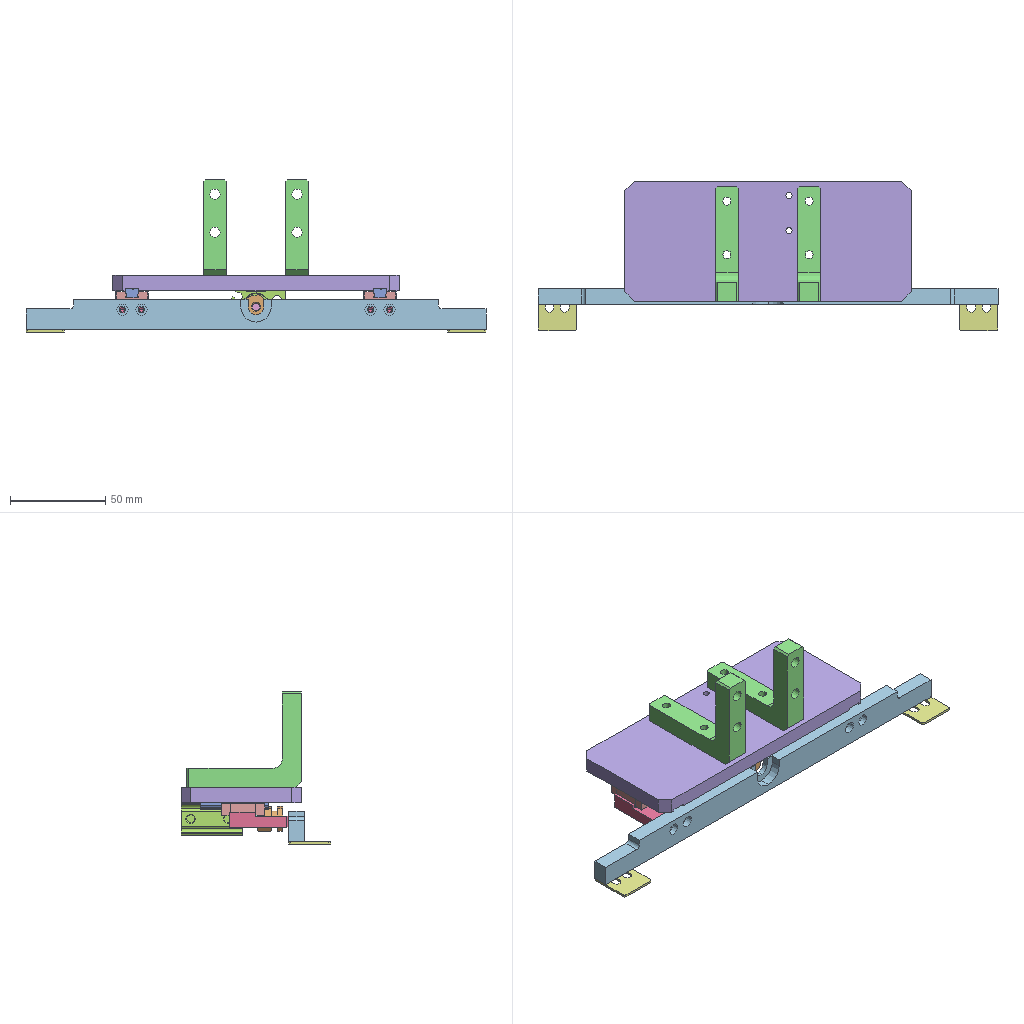Assembly | SolidWorks | 9 different items | 14 placed | box 241 x 78 x 80 mm
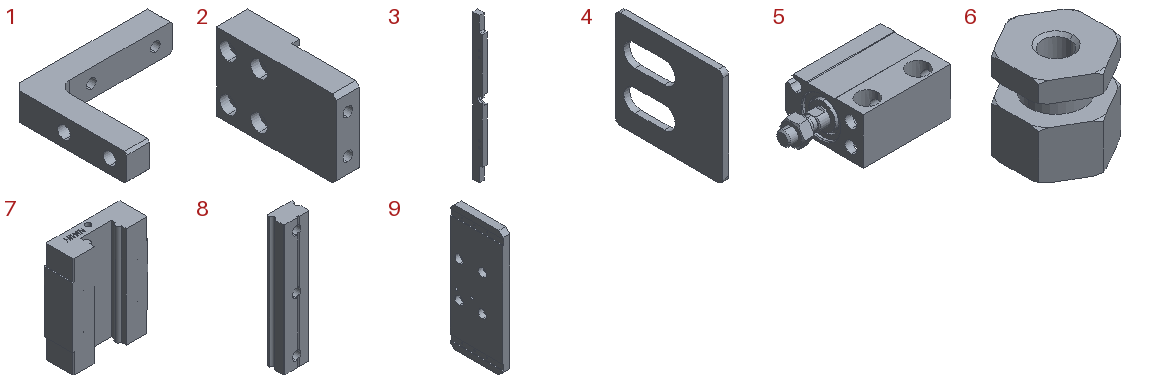Parts list (item | quantity | size | volume | features):
1 | x2 | 60 x 50 x 12 mm | 11238 mm3 | features HoleWzd 2, Chamfer 1, Extrusion 1, Fillet 1
2 | x2 | 8 x 31 x 20 mm | 3513 mm3 | features HoleWzd 2, Chamfer 1, Cut 1, Extrusion 1, ICE 1
3 | x1 | 8 x 16 x 241 mm | 26977 mm3 | features HoleWzd 2, ICE 2, Cut 1, Extrusion 1
4 | x2 | 1.2 x 22 x 20 mm | 424 mm3 | features Fillet 1, FlatPattern 1, HoleWzd 1, SMBaseFlange 1, SheetMetal 1
5 | x1 | 46 x 28.5 x 17 mm | 11423 mm3 | features BaseBody 3
6 | x1 | 12 x 13.856 x 13 mm | 1220 mm3 | features BaseBody 1
7 | x2 | 17 x 6.5 x 22.5 mm | 1833 mm3 | features BaseBody 1, HoleWzd 1
8 | x2 | 7 x 4.8 x 36 mm | 1017 mm3 | features ICE 2, Extrusion 1, HoleWzd 1, LPattern 1
9 | x1 | 8 x 63 x 150 mm | 72107 mm3 | features HoleWzd 3, Chamfer 1, Extrusion 1, ICE 1
Mates (type | each side: item.copy, entity, surface, feature):
Width | 7.1 face plane Input1 | 7.1 face plane Input1 | 8.1 face plane Boss-Extrude1 | 8.1 face plane Boss-Extrude1
Coincident | 8.1 face plane Boss-Extrude1 | 7.1 face plane Input1
Coincident | 7.1 face plane Input1 | 2.1 face plane Boss-Extrude1
Width | 7.1 face plane Input1 | 7.1 face plane Input1 | 2.1 face plane Boss-Extrude1 | 2.1 face plane Boss-Extrude1
LimitDistanceDim | 7.2 face plane Input1 | 8.2 face plane Cut-Extrude2
Coincident | 8.2 face plane Boss-Extrude1 | 7.2 face plane Input1
Width | 7.2 face plane Input1 | 7.2 face plane Input1 | 8.2 face plane Boss-Extrude1 | 8.2 face plane Boss-Extrude1
Coincident | 8.1 face plane Cut-Extrude2 | 8.2 face plane Cut-Extrude2
Concentric | 5.1 face cylinder _MU12X10SB_rod-1-solid1 | 6.1 face cylinder Input1
DistanceDim | 6.1 face plane Input1 | 5.1 face plane _12_nut-1-solid1
Coincident | 5.1 face plane _MU12X10S_body-1-solid1 | 9.1 face plane Boss-Extrude1 | 2 times
Coincident | 2.1 face plane Boss-Extrude1 | 9.1 face plane Boss-Extrude1
Coincident | 9.1 face plane Boss-Extrude1 | 1.1 face plane Boss-Extrude1 | 2 times
Coincident | 9.1 face plane Boss-Extrude1 | 1.2 face plane Boss-Extrude1
DistanceDim | 1.1 face plane Boss-Extrude1 | 1.2 face plane Boss-Extrude1
Width | 9.1 face plane Boss-Extrude1 | 9.1 face plane Boss-Extrude1 | 1.1 face plane Boss-Extrude1 | 1.2 face plane Boss-Extrude1
Coincident | 1.1 face plane Boss-Extrude1 | 1.2 face plane Boss-Extrude1
Width | 9.1 face plane Boss-Extrude1 | 9.1 face plane Boss-Extrude1 | 8.2 face plane Boss-Extrude1 | 8.1 face plane Boss-Extrude1
Coincident | 2.2 face plane Boss-Extrude1 | 7.2 face plane Input1
Width | 2.2 face plane Boss-Extrude1 | 2.2 face plane Boss-Extrude1 | 7.2 face plane Input1 | 7.2 face plane Input1
DistanceDim | 5.1 face plane _MU12X10S_body-1-solid1 | 9.1 face plane Boss-Extrude1
DistanceDim | 8.1 face plane Cut-Extrude2 | 9.1 face plane Boss-Extrude1
Concentric | 3.1 face cylinder Cut-Extrude2 | 6.1 face cylinder Input1
Coincident | 2.1 face plane Boss-Extrude1 | 2.2 face plane Boss-Extrude1
Coincident | 3.1 face plane Boss-Extrude2 | 2.1 face plane Boss-Extrude1
LimitDistanceDim | 7.1 face plane Input1 | 8.1 face plane Cut-Extrude2
Coincident | 3.1 face plane Boss-Extrude2 | 4.1 face plane Base-Flange1 | 3 times
Coincident | 3.1 face plane Boss-Extrude2 | 4.2 face plane Base-Flange1 | 3 times
Parallel | 3.1 face plane Boss-Extrude2 | 2.2 face plane Boss-Extrude1
Coincident | 8.1 face plane Boss-Extrude1 | 9.1 face plane Cut-Extrude1
Coincident | 8.2 face plane Boss-Extrude1 | 9.1 face plane Cut-Extrude1
DistanceDim | 2.1 face plane Boss-Extrude1 | 7.1 face plane Input1
DistanceDim | 2.2 face plane Boss-Extrude1 | 7.2 face plane Input1